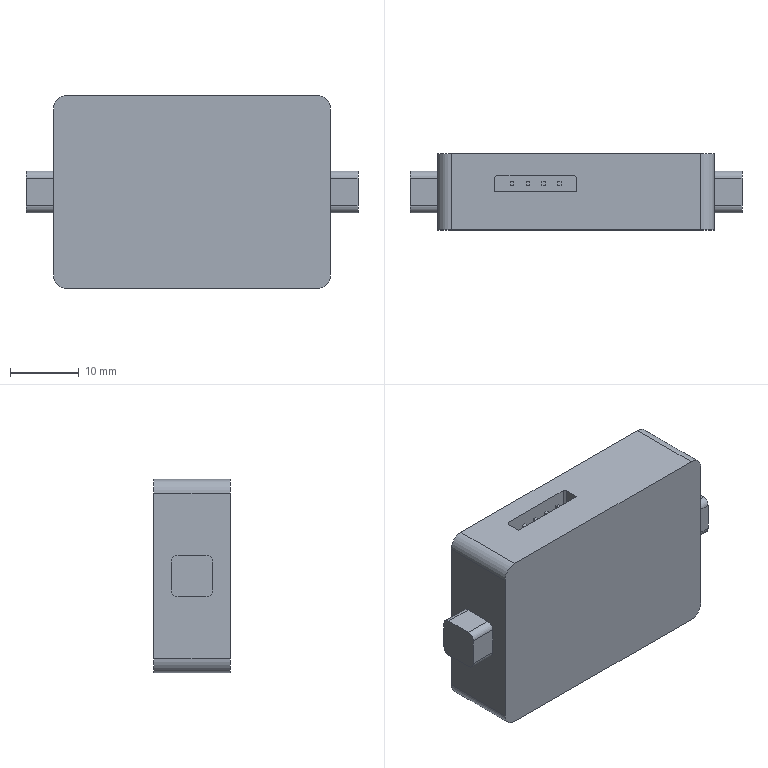Part | SolidWorks | features ICE 7, Fillet 2, Chamfer 1, Extrusion 1 | 1 solid | 55 faces | box 48.33 x 11.1 x 28.16 mm | volume 12571 mm3 | plane 43 | cylinder 12 | commonest cylinder face diameters 2 x8 4 x4